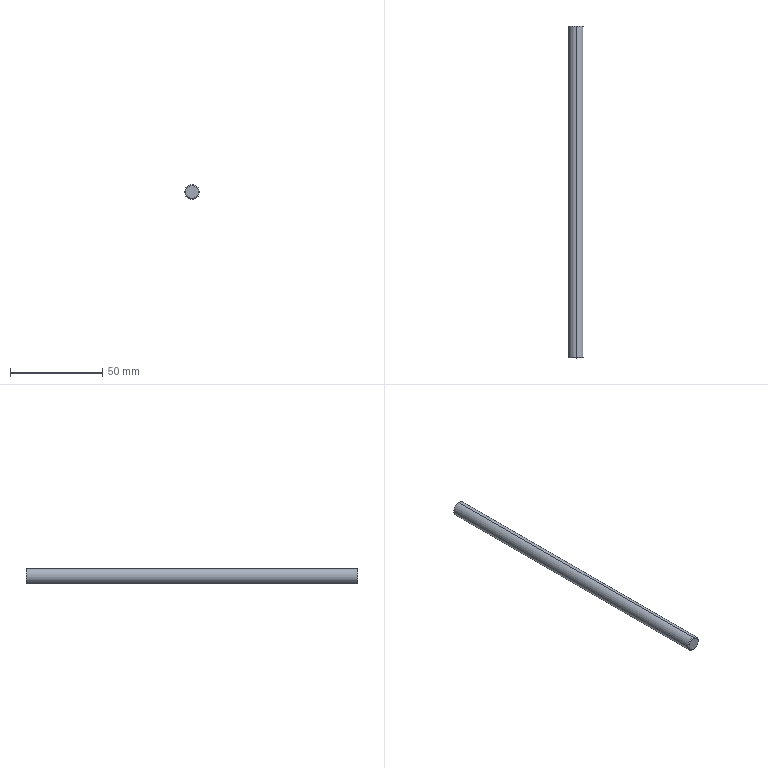Part | STEP file | 1 solid | 10 faces | box 8 x 180 x 8 mm | volume 8853 mm3 | cone 4 | cylinder 4 | plane 2 | commonest cylinder face diameters 3.3 x2 8 x2
STEP:
#1=CARTESIAN_POINT('',(0.,0.,0.));
#2=DIRECTION('',(0.,0.,1.));
#3=DIRECTION('',(1.,0.,0.));
#4=AXIS2_PLACEMENT_3D('',#1,#2,#3);
#5=CARTESIAN_POINT('',(0.,0.,-3.5));
#6=VERTEX_POINT('',#5);
#7=CARTESIAN_POINT('',(0.,0.5,-4.));
#8=VERTEX_POINT('',#7);
#9=CARTESIAN_POINT('',(0.,0.5,-4.));
#10=DIRECTION('',(0.,0.7071,-0.7071));
#11=VECTOR('',#10,1.);
#12=LINE('',#9,#11);
#13=CARTESIAN_POINT('',(0.,0.5,0.));
#14=DIRECTION('',(0.,1.,0.));
#15=DIRECTION('',(0.,0.,1.));
#16=AXIS2_PLACEMENT_3D('',#13,#14,#15);
#17=CONICAL_SURFACE('',#16,4.,0.7854);
#18=CARTESIAN_POINT('',(3.142,0.));
#19=DIRECTION('',(0.,1.));
#20=VECTOR('',#19,1.);
#21=LINE('',#18,#20);
#22=(GEOMETRIC_REPRESENTATION_CONTEXT(2)PARAMETRIC_REPRESENTATION_CONTEXT()REPRESENTATION_CONTEXT('',''));
#23=DEFINITIONAL_REPRESENTATION('',(#21),#22);
#24=PCURVE('',#17,#23);
#25=CARTESIAN_POINT('',(0.,0.5,0.));
#26=DIRECTION('',(0.,1.,0.));
#27=DIRECTION('',(0.,0.,1.));
#28=AXIS2_PLACEMENT_3D('',#25,#26,#27);
#29=CONICAL_SURFACE('',#28,4.,0.7854);
#30=CARTESIAN_POINT('',(3.142,0.));
#31=DIRECTION('',(0.,1.));
#32=VECTOR('',#31,1.);
#33=LINE('',#30,#32);
#34=(GEOMETRIC_REPRESENTATION_CONTEXT(2)PARAMETRIC_REPRESENTATION_CONTEXT()REPRESENTATION_CONTEXT('',''));
#35=DEFINITIONAL_REPRESENTATION('',(#33),#34);
#36=PCURVE('',#29,#35);
#37=SURFACE_CURVE('',#12,(#24,#36),.PCURVE_S1.);
#38=EDGE_CURVE('',#6,#8,#37,.T.);
#39=ORIENTED_EDGE('',*,*,#38,.F.);
#40=CARTESIAN_POINT('',(0.,0.,3.5));
#41=VERTEX_POINT('',#40);
#42=CARTESIAN_POINT('',(0.,0.,0.));
#43=DIRECTION('',(0.,-1.,0.));
#44=DIRECTION('',(0.,0.,1.));
#45=AXIS2_PLACEMENT_3D('',#42,#43,#44);
#46=CIRCLE('',#45,3.5);
#47=CARTESIAN_POINT('',(6.283,-0.5));
#48=DIRECTION('',(-1.,0.));
#49=VECTOR('',#48,1.);
#50=LINE('',#47,#49);
#51=(GEOMETRIC_REPRESENTATION_CONTEXT(2)PARAMETRIC_REPRESENTATION_CONTEXT()REPRESENTATION_CONTEXT('',''));
#52=DEFINITIONAL_REPRESENTATION('',(#50),#51);
#53=PCURVE('',#17,#52);
#54=CARTESIAN_POINT('',(0.,0.,0.));
#55=DIRECTION('',(0.,1.,0.));
#56=DIRECTION('',(1.,0.,0.));
#57=AXIS2_PLACEMENT_3D('',#54,#55,#56);
#58=PLANE('',#57);
#59=CARTESIAN_POINT('',(0.,-3.5));
#60=CARTESIAN_POINT('',(-6.062,-3.5));
#61=CARTESIAN_POINT('',(-3.031,1.75));
#62=CARTESIAN_POINT('',(0.,7.));
#63=CARTESIAN_POINT('',(3.031,1.75));
#64=CARTESIAN_POINT('',(6.062,-3.5));
#65=CARTESIAN_POINT('',(0.,-3.5));
#66=(BOUNDED_CURVE()B_SPLINE_CURVE(2,(#59,#60,#61,#62,#63,#64,#65),.UNSPECIFIED.,.T.,.F.)B_SPLINE_CURVE_WITH_KNOTS((1,2,2,2,2,1),(-2.094,0.,2.094,4.189,6.283,8.378),.UNSPECIFIED.)CURVE()GEOMETRIC_REPRESENTATION_ITEM()RATIONAL_B_SPLINE_CURVE((1.,0.5,1.,0.5,1.,0.5,1.))REPRESENTATION_ITEM(''));
#67=(GEOMETRIC_REPRESENTATION_CONTEXT(2)PARAMETRIC_REPRESENTATION_CONTEXT()REPRESENTATION_CONTEXT('',''));
#68=DEFINITIONAL_REPRESENTATION('',(#66),#67);
#69=PCURVE('',#58,#68);
#70=SURFACE_CURVE('',#46,(#53,#69),.PCURVE_S1.);
#71=EDGE_CURVE('',#41,#6,#70,.T.);
#72=ORIENTED_EDGE('',*,*,#71,.F.);
#73=CARTESIAN_POINT('',(0.,0.5,4.));
#74=VERTEX_POINT('',#73);
#75=CARTESIAN_POINT('',(0.,0.5,4.));
#76=DIRECTION('',(0.,0.7071,0.7071));
#77=VECTOR('',#76,1.);
#78=LINE('',#75,#77);
#79=CARTESIAN_POINT('',(6.283,0.));
#80=DIRECTION('',(0.,1.));
#81=VECTOR('',#80,1.);
#82=LINE('',#79,#81);
#83=(GEOMETRIC_REPRESENTATION_CONTEXT(2)PARAMETRIC_REPRESENTATION_CONTEXT()REPRESENTATION_CONTEXT('',''));
#84=DEFINITIONAL_REPRESENTATION('',(#82),#83);
#85=PCURVE('',#17,#84);
#86=CARTESIAN_POINT('',(0.,0.));
#87=DIRECTION('',(0.,1.));
#88=VECTOR('',#87,1.);
#89=LINE('',#86,#88);
#90=(GEOMETRIC_REPRESENTATION_CONTEXT(2)PARAMETRIC_REPRESENTATION_CONTEXT()REPRESENTATION_CONTEXT('',''));
#91=DEFINITIONAL_REPRESENTATION('',(#89),#90);
#92=PCURVE('',#29,#91);
#93=SURFACE_CURVE('',#78,(#85,#92),.PCURVE_S1.);
#94=EDGE_CURVE('',#41,#74,#93,.T.);
#95=ORIENTED_EDGE('',*,*,#94,.T.);
#96=CARTESIAN_POINT('',(0.,0.5,0.));
#97=DIRECTION('',(0.,1.,0.));
#98=DIRECTION('',(0.,0.,1.));
#99=AXIS2_PLACEMENT_3D('',#96,#97,#98);
#100=CIRCLE('',#99,4.);
#101=CARTESIAN_POINT('',(0.,0.));
#102=DIRECTION('',(1.,0.));
#103=VECTOR('',#102,1.);
#104=LINE('',#101,#103);
#105=(GEOMETRIC_REPRESENTATION_CONTEXT(2)PARAMETRIC_REPRESENTATION_CONTEXT()REPRESENTATION_CONTEXT('',''));
#106=DEFINITIONAL_REPRESENTATION('',(#104),#105);
#107=PCURVE('',#17,#106);
#108=CARTESIAN_POINT('',(0.,180.,0.));
#109=DIRECTION('',(0.,-1.,0.));
#110=DIRECTION('',(0.,0.,-1.));
#111=AXIS2_PLACEMENT_3D('',#108,#109,#110);
#112=CYLINDRICAL_SURFACE('',#111,4.);
#113=CARTESIAN_POINT('',(9.425,179.5));
#114=DIRECTION('',(-1.,0.));
#115=VECTOR('',#114,1.);
#116=LINE('',#113,#115);
#117=(GEOMETRIC_REPRESENTATION_CONTEXT(2)PARAMETRIC_REPRESENTATION_CONTEXT()REPRESENTATION_CONTEXT('',''));
#118=DEFINITIONAL_REPRESENTATION('',(#116),#117);
#119=PCURVE('',#112,#118);
#120=SURFACE_CURVE('',#100,(#107,#119),.PCURVE_S1.);
#121=EDGE_CURVE('',#8,#74,#120,.T.);
#122=ORIENTED_EDGE('',*,*,#121,.F.);
#123=EDGE_LOOP('',(#39,#72,#95,#122));
#124=FACE_BOUND('',#123,.T.);
#125=ADVANCED_FACE('',(#124),#17,.T.);
#126=CARTESIAN_POINT('',(0.,180.,1.65));
#127=VERTEX_POINT('',#126);
#128=CARTESIAN_POINT('',(0.,180.,-1.65));
#129=VERTEX_POINT('',#128);
#130=CARTESIAN_POINT('',(0.,180.,0.));
#131=DIRECTION('',(0.,1.,0.));
#132=DIRECTION('',(0.,0.,1.));
#133=AXIS2_PLACEMENT_3D('',#130,#131,#132);
#134=CIRCLE('',#133,1.65);
#135=CARTESIAN_POINT('',(0.,180.,0.));
#136=DIRECTION('',(0.,1.,0.));
#137=DIRECTION('',(0.,0.,1.));
#138=AXIS2_PLACEMENT_3D('',#135,#136,#137);
#139=CYLINDRICAL_SURFACE('',#138,1.65);
#140=CARTESIAN_POINT('',(0.,0.));
#141=DIRECTION('',(1.,0.));
#142=VECTOR('',#141,1.);
#143=LINE('',#140,#142);
#144=(GEOMETRIC_REPRESENTATION_CONTEXT(2)PARAMETRIC_REPRESENTATION_CONTEXT()REPRESENTATION_CONTEXT('',''));
#145=DEFINITIONAL_REPRESENTATION('',(#143),#144);
#146=PCURVE('',#139,#145);
#147=CARTESIAN_POINT('',(0.,180.,0.));
#148=DIRECTION('',(0.,1.,0.));
#149=DIRECTION('',(1.,0.,0.));
#150=AXIS2_PLACEMENT_3D('',#147,#148,#149);
#151=PLANE('',#150);
#152=CARTESIAN_POINT('',(0.,0.));
#153=DIRECTION('',(0.,-1.));
#154=AXIS2_PLACEMENT_2D('',#152,#153);
#155=CIRCLE('',#154,1.65);
#156=(GEOMETRIC_REPRESENTATION_CONTEXT(2)PARAMETRIC_REPRESENTATION_CONTEXT()REPRESENTATION_CONTEXT('',''));
#157=DEFINITIONAL_REPRESENTATION('',(#155),#156);
#158=PCURVE('',#151,#157);
#159=SURFACE_CURVE('',#134,(#146,#158),.PCURVE_S1.);
#160=EDGE_CURVE('',#127,#129,#159,.T.);
#161=ORIENTED_EDGE('',*,*,#160,.F.);
#162=CARTESIAN_POINT('',(0.,157.9,1.65));
#163=VERTEX_POINT('',#162);
#164=CARTESIAN_POINT('',(0.,180.,1.65));
#165=DIRECTION('',(0.,1.,0.));
#166=VECTOR('',#165,1.);
#167=LINE('',#164,#166);
#168=CARTESIAN_POINT('',(0.,0.));
#169=DIRECTION('',(0.,1.));
#170=VECTOR('',#169,1.);
#171=LINE('',#168,#170);
#172=(GEOMETRIC_REPRESENTATION_CONTEXT(2)PARAMETRIC_REPRESENTATION_CONTEXT()REPRESENTATION_CONTEXT('',''));
#173=DEFINITIONAL_REPRESENTATION('',(#171),#172);
#174=PCURVE('',#139,#173);
#175=CARTESIAN_POINT('',(0.,180.,0.));
#176=DIRECTION('',(0.,1.,0.));
#177=DIRECTION('',(0.,0.,1.));
#178=AXIS2_PLACEMENT_3D('',#175,#176,#177);
#179=CYLINDRICAL_SURFACE('',#178,1.65);
#180=CARTESIAN_POINT('',(6.283,0.));
#181=DIRECTION('',(0.,1.));
#182=VECTOR('',#181,1.);
#183=LINE('',#180,#182);
#184=(GEOMETRIC_REPRESENTATION_CONTEXT(2)PARAMETRIC_REPRESENTATION_CONTEXT()REPRESENTATION_CONTEXT('',''));
#185=DEFINITIONAL_REPRESENTATION('',(#183),#184);
#186=PCURVE('',#179,#185);
#187=SURFACE_CURVE('',#167,(#174,#186),.PCURVE_S1.);
#188=EDGE_CURVE('',#163,#127,#187,.T.);
#189=ORIENTED_EDGE('',*,*,#188,.F.);
#190=CARTESIAN_POINT('',(0.,157.9,-1.65));
#191=VERTEX_POINT('',#190);
#192=CARTESIAN_POINT('',(0.,157.9,0.));
#193=DIRECTION('',(0.,1.,0.));
#194=DIRECTION('',(0.,0.,1.));
#195=AXIS2_PLACEMENT_3D('',#192,#193,#194);
#196=CIRCLE('',#195,1.65);
#197=CARTESIAN_POINT('',(0.,-22.1));
#198=DIRECTION('',(1.,0.));
#199=VECTOR('',#198,1.);
#200=LINE('',#197,#199);
#201=(GEOMETRIC_REPRESENTATION_CONTEXT(2)PARAMETRIC_REPRESENTATION_CONTEXT()REPRESENTATION_CONTEXT('',''));
#202=DEFINITIONAL_REPRESENTATION('',(#200),#201);
#203=PCURVE('',#139,#202);
#204=CARTESIAN_POINT('',(0.,157.9,0.));
#205=DIRECTION('',(0.,1.,0.));
#206=DIRECTION('',(0.,0.,1.));
#207=AXIS2_PLACEMENT_3D('',#204,#205,#206);
#208=CONICAL_SURFACE('',#207,1.65,1.03);
#209=CARTESIAN_POINT('',(0.,0.));
#210=DIRECTION('',(1.,0.));
#211=VECTOR('',#210,1.);
#212=LINE('',#209,#211);
#213=(GEOMETRIC_REPRESENTATION_CONTEXT(2)PARAMETRIC_REPRESENTATION_CONTEXT()REPRESENTATION_CONTEXT('',''));
#214=DEFINITIONAL_REPRESENTATION('',(#212),#213);
#215=PCURVE('',#208,#214);
#216=SURFACE_CURVE('',#196,(#203,#215),.PCURVE_S1.);
#217=EDGE_CURVE('',#163,#191,#216,.T.);
#218=ORIENTED_EDGE('',*,*,#217,.T.);
#219=CARTESIAN_POINT('',(0.,180.,-1.65));
#220=DIRECTION('',(0.,1.,0.));
#221=VECTOR('',#220,1.);
#222=LINE('',#219,#221);
#223=CARTESIAN_POINT('',(3.142,0.));
#224=DIRECTION('',(0.,1.));
#225=VECTOR('',#224,1.);
#226=LINE('',#223,#225);
#227=(GEOMETRIC_REPRESENTATION_CONTEXT(2)PARAMETRIC_REPRESENTATION_CONTEXT()REPRESENTATION_CONTEXT('',''));
#228=DEFINITIONAL_REPRESENTATION('',(#226),#227);
#229=PCURVE('',#139,#228);
#230=CARTESIAN_POINT('',(3.142,0.));
#231=DIRECTION('',(0.,1.));
#232=VECTOR('',#231,1.);
#233=LINE('',#230,#232);
#234=(GEOMETRIC_REPRESENTATION_CONTEXT(2)PARAMETRIC_REPRESENTATION_CONTEXT()REPRESENTATION_CONTEXT('',''));
#235=DEFINITIONAL_REPRESENTATION('',(#233),#234);
#236=PCURVE('',#179,#235);
#237=SURFACE_CURVE('',#222,(#229,#236),.PCURVE_S1.);
#238=EDGE_CURVE('',#191,#129,#237,.T.);
#239=ORIENTED_EDGE('',*,*,#238,.T.);
#240=EDGE_LOOP('',(#161,#189,#218,#239));
#241=FACE_BOUND('',#240,.F.);
#242=ADVANCED_FACE('',(#241),#139,.F.);
#243=ORIENTED_EDGE('',*,*,#217,.F.);
#244=CARTESIAN_POINT('',(0.,156.909,0.));
#245=VERTEX_POINT('',#244);
#246=CARTESIAN_POINT('',(0.,157.9,1.65));
#247=DIRECTION('',(0.,0.515,0.8572));
#248=VECTOR('',#247,1.);
#249=LINE('',#246,#248);
#250=CARTESIAN_POINT('',(0.,0.));
#251=DIRECTION('',(0.,1.));
#252=VECTOR('',#251,1.);
#253=LINE('',#250,#252);
#254=(GEOMETRIC_REPRESENTATION_CONTEXT(2)PARAMETRIC_REPRESENTATION_CONTEXT()REPRESENTATION_CONTEXT('',''));
#255=DEFINITIONAL_REPRESENTATION('',(#253),#254);
#256=PCURVE('',#208,#255);
#257=CARTESIAN_POINT('',(0.,157.9,0.));
#258=DIRECTION('',(0.,1.,0.));
#259=DIRECTION('',(0.,0.,1.));
#260=AXIS2_PLACEMENT_3D('',#257,#258,#259);
#261=CONICAL_SURFACE('',#260,1.65,1.03);
#262=CARTESIAN_POINT('',(6.283,0.));
#263=DIRECTION('',(0.,1.));
#264=VECTOR('',#263,1.);
#265=LINE('',#262,#264);
#266=(GEOMETRIC_REPRESENTATION_CONTEXT(2)PARAMETRIC_REPRESENTATION_CONTEXT()REPRESENTATION_CONTEXT('',''));
#267=DEFINITIONAL_REPRESENTATION('',(#265),#266);
#268=PCURVE('',#261,#267);
#269=SURFACE_CURVE('',#249,(#256,#268),.PCURVE_S1.);
#270=EDGE_CURVE('',#245,#163,#269,.T.);
#271=ORIENTED_EDGE('',*,*,#270,.F.);
#272=CARTESIAN_POINT('',(0.,157.9,-1.65));
#273=DIRECTION('',(0.,0.515,-0.8572));
#274=VECTOR('',#273,1.);
#275=LINE('',#272,#274);
#276=CARTESIAN_POINT('',(3.142,0.));
#277=DIRECTION('',(0.,1.));
#278=VECTOR('',#277,1.);
#279=LINE('',#276,#278);
#280=(GEOMETRIC_REPRESENTATION_CONTEXT(2)PARAMETRIC_REPRESENTATION_CONTEXT()REPRESENTATION_CONTEXT('',''));
#281=DEFINITIONAL_REPRESENTATION('',(#279),#280);
#282=PCURVE('',#208,#281);
#283=CARTESIAN_POINT('',(3.142,0.));
#284=DIRECTION('',(0.,1.));
#285=VECTOR('',#284,1.);
#286=LINE('',#283,#285);
#287=(GEOMETRIC_REPRESENTATION_CONTEXT(2)PARAMETRIC_REPRESENTATION_CONTEXT()REPRESENTATION_CONTEXT('',''));
#288=DEFINITIONAL_REPRESENTATION('',(#286),#287);
#289=PCURVE('',#261,#288);
#290=SURFACE_CURVE('',#275,(#282,#289),.PCURVE_S1.);
#291=EDGE_CURVE('',#245,#191,#290,.T.);
#292=ORIENTED_EDGE('',*,*,#291,.T.);
#293=EDGE_LOOP('',(#243,#271,#292));
#294=FACE_BOUND('',#293,.F.);
#295=ADVANCED_FACE('',(#294),#208,.F.);
#296=ORIENTED_EDGE('',*,*,#71,.T.);
#297=CARTESIAN_POINT('',(0.,0.,0.));
#298=DIRECTION('',(0.,-1.,0.));
#299=DIRECTION('',(0.,0.,1.));
#300=AXIS2_PLACEMENT_3D('',#297,#298,#299);
#301=CIRCLE('',#300,3.5);
#302=CARTESIAN_POINT('',(0.,-3.5));
#303=CARTESIAN_POINT('',(-6.062,-3.5));
#304=CARTESIAN_POINT('',(-3.031,1.75));
#305=CARTESIAN_POINT('',(0.,7.));
#306=CARTESIAN_POINT('',(3.031,1.75));
#307=CARTESIAN_POINT('',(6.062,-3.5));
#308=CARTESIAN_POINT('',(0.,-3.5));
#309=(BOUNDED_CURVE()B_SPLINE_CURVE(2,(#302,#303,#304,#305,#306,#307,#308),.UNSPECIFIED.,.T.,.F.)B_SPLINE_CURVE_WITH_KNOTS((1,2,2,2,2,1),(-2.094,0.,2.094,4.189,6.283,8.378),.UNSPECIFIED.)CURVE()GEOMETRIC_REPRESENTATION_ITEM()RATIONAL_B_SPLINE_CURVE((1.,0.5,1.,0.5,1.,0.5,1.))REPRESENTATION_ITEM(''));
#310=(GEOMETRIC_REPRESENTATION_CONTEXT(2)PARAMETRIC_REPRESENTATION_CONTEXT()REPRESENTATION_CONTEXT('',''));
#311=DEFINITIONAL_REPRESENTATION('',(#309),#310);
#312=PCURVE('',#58,#311);
#313=CARTESIAN_POINT('',(6.283,-0.5));
#314=DIRECTION('',(-1.,0.));
#315=VECTOR('',#314,1.);
#316=LINE('',#313,#315);
#317=(GEOMETRIC_REPRESENTATION_CONTEXT(2)PARAMETRIC_REPRESENTATION_CONTEXT()REPRESENTATION_CONTEXT('',''));
#318=DEFINITIONAL_REPRESENTATION('',(#316),#317);
#319=PCURVE('',#29,#318);
#320=SURFACE_CURVE('',#301,(#312,#319),.PCURVE_S1.);
#321=EDGE_CURVE('',#6,#41,#320,.T.);
#322=ORIENTED_EDGE('',*,*,#321,.T.);
#323=EDGE_LOOP('',(#296,#322));
#324=FACE_BOUND('',#323,.T.);
#325=ADVANCED_FACE('',(#324),#58,.F.);
#326=ORIENTED_EDGE('',*,*,#160,.F.);
#327=CARTESIAN_POINT('',(0.,180.,0.));
#328=DIRECTION('',(0.,1.,0.));
#329=DIRECTION('',(0.,0.,1.));
#330=AXIS2_PLACEMENT_3D('',#327,#328,#329);
#331=CIRCLE('',#330,1.65);
#332=CARTESIAN_POINT('',(0.,0.));
#333=DIRECTION('',(0.,-1.));
#334=AXIS2_PLACEMENT_2D('',#332,#333);
#335=CIRCLE('',#334,1.65);
#336=(GEOMETRIC_REPRESENTATION_CONTEXT(2)PARAMETRIC_REPRESENTATION_CONTEXT()REPRESENTATION_CONTEXT('',''));
#337=DEFINITIONAL_REPRESENTATION('',(#335),#336);
#338=PCURVE('',#151,#337);
#339=CARTESIAN_POINT('',(0.,0.));
#340=DIRECTION('',(1.,0.));
#341=VECTOR('',#340,1.);
#342=LINE('',#339,#341);
#343=(GEOMETRIC_REPRESENTATION_CONTEXT(2)PARAMETRIC_REPRESENTATION_CONTEXT()REPRESENTATION_CONTEXT('',''));
#344=DEFINITIONAL_REPRESENTATION('',(#342),#343);
#345=PCURVE('',#179,#344);
#346=SURFACE_CURVE('',#331,(#338,#345),.PCURVE_S1.);
#347=EDGE_CURVE('',#129,#127,#346,.T.);
#348=ORIENTED_EDGE('',*,*,#347,.F.);
#349=EDGE_LOOP('',(#326,#348));
#350=FACE_BOUND('',#349,.T.);
#351=CARTESIAN_POINT('',(0.,180.,-4.));
#352=VERTEX_POINT('',#351);
#353=CARTESIAN_POINT('',(0.,180.,4.));
#354=VERTEX_POINT('',#353);
#355=CARTESIAN_POINT('',(0.,180.,0.));
#356=DIRECTION('',(0.,1.,0.));
#357=DIRECTION('',(0.,0.,1.));
#358=AXIS2_PLACEMENT_3D('',#355,#356,#357);
#359=CIRCLE('',#358,4.);
#360=CARTESIAN_POINT('',(0.,0.));
#361=DIRECTION('',(0.,-1.));
#362=AXIS2_PLACEMENT_2D('',#360,#361);
#363=CIRCLE('',#362,4.);
#364=(GEOMETRIC_REPRESENTATION_CONTEXT(2)PARAMETRIC_REPRESENTATION_CONTEXT()REPRESENTATION_CONTEXT('',''));
#365=DEFINITIONAL_REPRESENTATION('',(#363),#364);
#366=PCURVE('',#151,#365);
#367=CARTESIAN_POINT('',(9.425,0.));
#368=DIRECTION('',(-1.,0.));
#369=VECTOR('',#368,1.);
#370=LINE('',#367,#369);
#371=(GEOMETRIC_REPRESENTATION_CONTEXT(2)PARAMETRIC_REPRESENTATION_CONTEXT()REPRESENTATION_CONTEXT('',''));
#372=DEFINITIONAL_REPRESENTATION('',(#370),#371);
#373=PCURVE('',#112,#372);
#374=SURFACE_CURVE('',#359,(#366,#373),.PCURVE_S1.);
#375=EDGE_CURVE('',#352,#354,#374,.T.);
#376=ORIENTED_EDGE('',*,*,#375,.T.);
#377=CARTESIAN_POINT('',(0.,180.,0.));
#378=DIRECTION('',(0.,1.,0.));
#379=DIRECTION('',(0.,0.,1.));
#380=AXIS2_PLACEMENT_3D('',#377,#378,#379);
#381=CIRCLE('',#380,4.);
#382=CARTESIAN_POINT('',(0.,0.));
#383=DIRECTION('',(0.,-1.));
#384=AXIS2_PLACEMENT_2D('',#382,#383);
#385=CIRCLE('',#384,4.);
#386=(GEOMETRIC_REPRESENTATION_CONTEXT(2)PARAMETRIC_REPRESENTATION_CONTEXT()REPRESENTATION_CONTEXT('',''));
#387=DEFINITIONAL_REPRESENTATION('',(#385),#386);
#388=PCURVE('',#151,#387);
#389=CARTESIAN_POINT('',(0.,180.,0.));
#390=DIRECTION('',(0.,-1.,0.));
#391=DIRECTION('',(0.,0.,-1.));
#392=AXIS2_PLACEMENT_3D('',#389,#390,#391);
#393=CYLINDRICAL_SURFACE('',#392,4.);
#394=CARTESIAN_POINT('',(3.142,0.));
#395=DIRECTION('',(-1.,0.));
#396=VECTOR('',#395,1.);
#397=LINE('',#394,#396);
#398=(GEOMETRIC_REPRESENTATION_CONTEXT(2)PARAMETRIC_REPRESENTATION_CONTEXT()REPRESENTATION_CONTEXT('',''));
#399=DEFINITIONAL_REPRESENTATION('',(#397),#398);
#400=PCURVE('',#393,#399);
#401=SURFACE_CURVE('',#381,(#388,#400),.PCURVE_S1.);
#402=EDGE_CURVE('',#354,#352,#401,.T.);
#403=ORIENTED_EDGE('',*,*,#402,.T.);
#404=EDGE_LOOP('',(#376,#403));
#405=FACE_BOUND('',#404,.T.);
#406=ADVANCED_FACE('',(#350,#405),#151,.T.);
#407=CARTESIAN_POINT('',(0.,180.,4.));
#408=DIRECTION('',(0.,-1.,0.));
#409=VECTOR('',#408,1.);
#410=LINE('',#407,#409);
#411=CARTESIAN_POINT('',(3.142,0.));
#412=DIRECTION('',(0.,1.));
#413=VECTOR('',#412,1.);
#414=LINE('',#411,#413);
#415=(GEOMETRIC_REPRESENTATION_CONTEXT(2)PARAMETRIC_REPRESENTATION_CONTEXT()REPRESENTATION_CONTEXT('',''));
#416=DEFINITIONAL_REPRESENTATION('',(#414),#415);
#417=PCURVE('',#112,#416);
#418=CARTESIAN_POINT('',(3.142,0.));
#419=DIRECTION('',(0.,1.));
#420=VECTOR('',#419,1.);
#421=LINE('',#418,#420);
#422=(GEOMETRIC_REPRESENTATION_CONTEXT(2)PARAMETRIC_REPRESENTATION_CONTEXT()REPRESENTATION_CONTEXT('',''));
#423=DEFINITIONAL_REPRESENTATION('',(#421),#422);
#424=PCURVE('',#393,#423);
#425=SURFACE_CURVE('',#410,(#417,#424),.PCURVE_S1.);
#426=EDGE_CURVE('',#354,#74,#425,.T.);
#427=ORIENTED_EDGE('',*,*,#426,.F.);
#428=ORIENTED_EDGE('',*,*,#375,.F.);
#429=CARTESIAN_POINT('',(0.,180.,-4.));
#430=DIRECTION('',(0.,-1.,0.));
#431=VECTOR('',#430,1.);
#432=LINE('',#429,#431);
#433=CARTESIAN_POINT('',(6.283,0.));
#434=DIRECTION('',(0.,1.));
#435=VECTOR('',#434,1.);
#436=LINE('',#433,#435);
#437=(GEOMETRIC_REPRESENTATION_CONTEXT(2)PARAMETRIC_REPRESENTATION_CONTEXT()REPRESENTATION_CONTEXT('',''));
#438=DEFINITIONAL_REPRESENTATION('',(#436),#437);
#439=PCURVE('',#112,#438);
#440=CARTESIAN_POINT('',(0.,0.));
#441=DIRECTION('',(0.,1.));
#442=VECTOR('',#441,1.);
#443=LINE('',#440,#442);
#444=(GEOMETRIC_REPRESENTATION_CONTEXT(2)PARAMETRIC_REPRESENTATION_CONTEXT()REPRESENTATION_CONTEXT('',''));
#445=DEFINITIONAL_REPRESENTATION('',(#443),#444);
#446=PCURVE('',#393,#445);
#447=SURFACE_CURVE('',#432,(#439,#446),.PCURVE_S1.);
#448=EDGE_CURVE('',#352,#8,#447,.T.);
#449=ORIENTED_EDGE('',*,*,#448,.T.);
#450=ORIENTED_EDGE('',*,*,#121,.T.);
#451=EDGE_LOOP('',(#427,#428,#449,#450));
#452=FACE_BOUND('',#451,.T.);
#453=ADVANCED_FACE('',(#452),#112,.T.);
#454=ORIENTED_EDGE('',*,*,#402,.F.);
#455=ORIENTED_EDGE('',*,*,#426,.T.);
#456=CARTESIAN_POINT('',(0.,0.5,0.));
#457=DIRECTION('',(0.,1.,0.));
#458=DIRECTION('',(0.,0.,1.));
#459=AXIS2_PLACEMENT_3D('',#456,#457,#458);
#460=CIRCLE('',#459,4.);
#461=CARTESIAN_POINT('',(3.142,179.5));
#462=DIRECTION('',(-1.,0.));
#463=VECTOR('',#462,1.);
#464=LINE('',#461,#463);
#465=(GEOMETRIC_REPRESENTATION_CONTEXT(2)PARAMETRIC_REPRESENTATION_CONTEXT()REPRESENTATION_CONTEXT('',''));
#466=DEFINITIONAL_REPRESENTATION('',(#464),#465);
#467=PCURVE('',#393,#466);
#468=CARTESIAN_POINT('',(0.,0.));
#469=DIRECTION('',(1.,0.));
#470=VECTOR('',#469,1.);
#471=LINE('',#468,#470);
#472=(GEOMETRIC_REPRESENTATION_CONTEXT(2)PARAMETRIC_REPRESENTATION_CONTEXT()REPRESENTATION_CONTEXT('',''));
#473=DEFINITIONAL_REPRESENTATION('',(#471),#472);
#474=PCURVE('',#29,#473);
#475=SURFACE_CURVE('',#460,(#467,#474),.PCURVE_S1.);
#476=EDGE_CURVE('',#74,#8,#475,.T.);
#477=ORIENTED_EDGE('',*,*,#476,.T.);
#478=ORIENTED_EDGE('',*,*,#448,.F.);
#479=EDGE_LOOP('',(#454,#455,#477,#478));
#480=FACE_BOUND('',#479,.T.);
#481=ADVANCED_FACE('',(#480),#393,.T.);
#482=CARTESIAN_POINT('',(0.,157.9,0.));
#483=DIRECTION('',(0.,1.,0.));
#484=DIRECTION('',(0.,0.,1.));
#485=AXIS2_PLACEMENT_3D('',#482,#483,#484);
#486=CIRCLE('',#485,1.65);
#487=CARTESIAN_POINT('',(0.,0.));
#488=DIRECTION('',(1.,0.));
#489=VECTOR('',#488,1.);
#490=LINE('',#487,#489);
#491=(GEOMETRIC_REPRESENTATION_CONTEXT(2)PARAMETRIC_REPRESENTATION_CONTEXT()REPRESENTATION_CONTEXT('',''));
#492=DEFINITIONAL_REPRESENTATION('',(#490),#491);
#493=PCURVE('',#261,#492);
#494=CARTESIAN_POINT('',(0.,-22.1));
#495=DIRECTION('',(1.,0.));
#496=VECTOR('',#495,1.);
#497=LINE('',#494,#496);
#498=(GEOMETRIC_REPRESENTATION_CONTEXT(2)PARAMETRIC_REPRESENTATION_CONTEXT()REPRESENTATION_CONTEXT('',''));
#499=DEFINITIONAL_REPRESENTATION('',(#497),#498);
#500=PCURVE('',#179,#499);
#501=SURFACE_CURVE('',#486,(#493,#500),.PCURVE_S1.);
#502=EDGE_CURVE('',#191,#163,#501,.T.);
#503=ORIENTED_EDGE('',*,*,#502,.F.);
#504=ORIENTED_EDGE('',*,*,#291,.F.);
#505=ORIENTED_EDGE('',*,*,#270,.T.);
#506=EDGE_LOOP('',(#503,#504,#505));
#507=FACE_BOUND('',#506,.F.);
#508=ADVANCED_FACE('',(#507),#261,.F.);
#509=ORIENTED_EDGE('',*,*,#188,.T.);
#510=ORIENTED_EDGE('',*,*,#347,.F.);
#511=ORIENTED_EDGE('',*,*,#238,.F.);
#512=ORIENTED_EDGE('',*,*,#502,.T.);
#513=EDGE_LOOP('',(#509,#510,#511,#512));
#514=FACE_BOUND('',#513,.F.);
#515=ADVANCED_FACE('',(#514),#179,.F.);
#516=ORIENTED_EDGE('',*,*,#321,.F.);
#517=ORIENTED_EDGE('',*,*,#38,.T.);
#518=ORIENTED_EDGE('',*,*,#476,.F.);
#519=ORIENTED_EDGE('',*,*,#94,.F.);
#520=EDGE_LOOP('',(#516,#517,#518,#519));
#521=FACE_BOUND('',#520,.T.);
#522=ADVANCED_FACE('',(#521),#29,.T.);
#523=CLOSED_SHELL('',(#125,#242,#295,#325,#406,#453,#481,#508,#515,#522));
#524=MANIFOLD_SOLID_BREP('',#523);
#525=(LENGTH_UNIT()NAMED_UNIT(*)SI_UNIT(.MILLI.,.METRE.));
#526=UNCERTAINTY_MEASURE_WITH_UNIT(LENGTH_MEASURE(0.0000001),#525,'','');
#527=(NAMED_UNIT(*)PLANE_ANGLE_UNIT()SI_UNIT($,.RADIAN.));
#528=(NAMED_UNIT(*)SI_UNIT($,.STERADIAN.)SOLID_ANGLE_UNIT());
#529=(GEOMETRIC_REPRESENTATION_CONTEXT(3)GLOBAL_UNCERTAINTY_ASSIGNED_CONTEXT((#526))GLOBAL_UNIT_ASSIGNED_CONTEXT((#525,#527,#528))REPRESENTATION_CONTEXT('',''));
#530=ADVANCED_BREP_SHAPE_REPRESENTATION('',(#4,#524),#529);